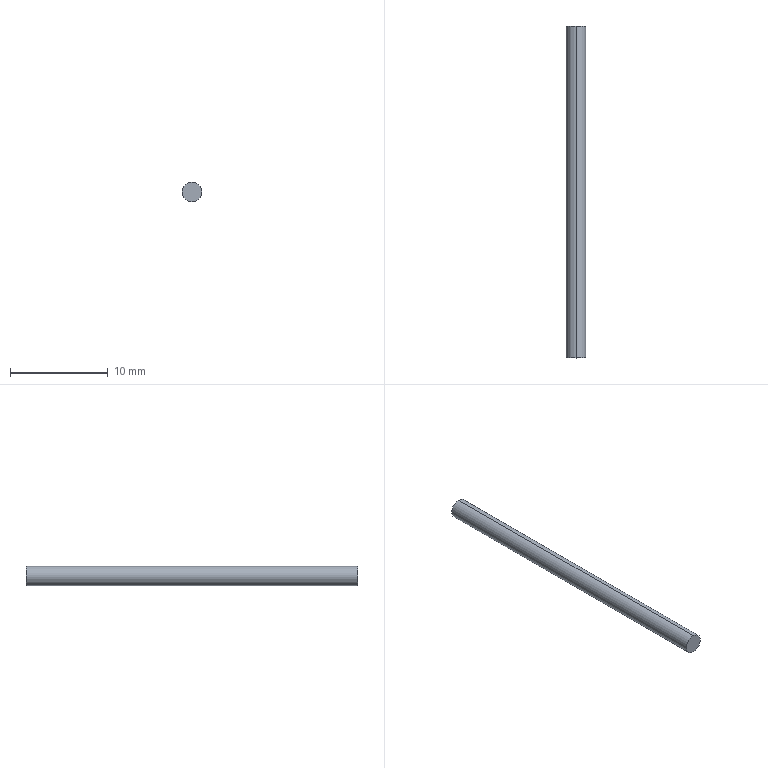Part | SolidWorks | features Extrusion 1 | 1 solid | 4 faces | box 2 x 34 x 2 mm | volume 106.814 mm3 | cylinder 2 | plane 2 | commonest cylinder face diameters 2 x2
STEP:
#1=CARTESIAN_POINT('',(0.,34.,1.));
#2=VERTEX_POINT('',#1);
#3=CARTESIAN_POINT('',(0.,34.,-1.));
#4=VERTEX_POINT('',#3);
#5=CARTESIAN_POINT('',(0.,34.,0.));
#6=DIRECTION('',(0.,1.,0.));
#7=DIRECTION('',(0.,0.,1.));
#8=AXIS2_PLACEMENT_3D('',#5,#6,#7);
#9=CIRCLE('',#8,1.);
#10=EDGE_CURVE('',#2,#4,#9,.T.);
#11=ORIENTED_EDGE('',*,*,#10,.F.);
#12=CARTESIAN_POINT('',(0.,0.,1.));
#13=VERTEX_POINT('',#12);
#14=CARTESIAN_POINT('',(0.,34.,1.));
#15=DIRECTION('',(0.,-1.,0.));
#16=VECTOR('',#15,1000.);
#17=LINE('',#14,#16);
#18=EDGE_CURVE('',#2,#13,#17,.T.);
#19=ORIENTED_EDGE('',*,*,#18,.T.);
#20=CARTESIAN_POINT('',(0.,0.,-1.));
#21=VERTEX_POINT('',#20);
#22=CARTESIAN_POINT('',(0.,0.,0.));
#23=DIRECTION('',(0.,1.,0.));
#24=DIRECTION('',(0.,0.,1.));
#25=AXIS2_PLACEMENT_3D('',#22,#23,#24);
#26=CIRCLE('',#25,1.);
#27=EDGE_CURVE('',#13,#21,#26,.T.);
#28=ORIENTED_EDGE('',*,*,#27,.T.);
#29=CARTESIAN_POINT('',(0.,34.,-1.));
#30=DIRECTION('',(0.,-1.,0.));
#31=VECTOR('',#30,1000.);
#32=LINE('',#29,#31);
#33=EDGE_CURVE('',#4,#21,#32,.T.);
#34=ORIENTED_EDGE('',*,*,#33,.F.);
#35=EDGE_LOOP('',(#11,#19,#28,#34));
#36=FACE_OUTER_BOUND('',#35,.T.);
#37=CARTESIAN_POINT('',(0.,34.,0.));
#38=DIRECTION('',(0.,-1.,0.));
#39=DIRECTION('',(0.,0.,-1.));
#40=AXIS2_PLACEMENT_3D('',#37,#38,#39);
#41=CYLINDRICAL_SURFACE('',#40,1.);
#42=ADVANCED_FACE('',(#36),#41,.T.);
#43=ORIENTED_EDGE('',*,*,#18,.F.);
#44=CARTESIAN_POINT('',(0.,34.,0.));
#45=DIRECTION('',(0.,1.,0.));
#46=DIRECTION('',(0.,0.,1.));
#47=AXIS2_PLACEMENT_3D('',#44,#45,#46);
#48=CIRCLE('',#47,1.);
#49=EDGE_CURVE('',#4,#2,#48,.T.);
#50=ORIENTED_EDGE('',*,*,#49,.F.);
#51=ORIENTED_EDGE('',*,*,#33,.T.);
#52=CARTESIAN_POINT('',(0.,0.,0.));
#53=DIRECTION('',(0.,1.,0.));
#54=DIRECTION('',(0.,0.,1.));
#55=AXIS2_PLACEMENT_3D('',#52,#53,#54);
#56=CIRCLE('',#55,1.);
#57=EDGE_CURVE('',#21,#13,#56,.T.);
#58=ORIENTED_EDGE('',*,*,#57,.T.);
#59=EDGE_LOOP('',(#43,#50,#51,#58));
#60=FACE_OUTER_BOUND('',#59,.T.);
#61=CARTESIAN_POINT('',(0.,34.,0.));
#62=DIRECTION('',(0.,-1.,0.));
#63=DIRECTION('',(0.,0.,-1.));
#64=AXIS2_PLACEMENT_3D('',#61,#62,#63);
#65=CYLINDRICAL_SURFACE('',#64,1.);
#66=ADVANCED_FACE('',(#60),#65,.T.);
#67=ORIENTED_EDGE('',*,*,#49,.T.);
#68=ORIENTED_EDGE('',*,*,#10,.T.);
#69=EDGE_LOOP('',(#67,#68));
#70=FACE_OUTER_BOUND('',#69,.T.);
#71=CARTESIAN_POINT('',(0.,34.,0.));
#72=DIRECTION('',(0.,1.,0.));
#73=DIRECTION('',(0.,0.,1.));
#74=AXIS2_PLACEMENT_3D('',#71,#72,#73);
#75=PLANE('',#74);
#76=ADVANCED_FACE('',(#70),#75,.T.);
#77=ORIENTED_EDGE('',*,*,#57,.F.);
#78=ORIENTED_EDGE('',*,*,#27,.F.);
#79=EDGE_LOOP('',(#77,#78));
#80=FACE_OUTER_BOUND('',#79,.T.);
#81=CARTESIAN_POINT('',(0.,0.,0.));
#82=DIRECTION('',(0.,1.,0.));
#83=DIRECTION('',(0.,0.,1.));
#84=AXIS2_PLACEMENT_3D('',#81,#82,#83);
#85=PLANE('',#84);
#86=ADVANCED_FACE('',(#80),#85,.F.);
#87=CLOSED_SHELL('',(#42,#66,#76,#86));
#88=MANIFOLD_SOLID_BREP('',#87);
#89=CARTESIAN_POINT('',(0.,0.,0.));
#90=DIRECTION('',(0.,0.,1.));
#91=DIRECTION('',(1.,0.,0.));
#92=AXIS2_PLACEMENT_3D('',#89,#90,#91);
#93=(LENGTH_UNIT()NAMED_UNIT(*)SI_UNIT(.MILLI.,.METRE.));
#94=UNCERTAINTY_MEASURE_WITH_UNIT(LENGTH_MEASURE(0.00001),#93,'','');
#95=(NAMED_UNIT(*)PLANE_ANGLE_UNIT()SI_UNIT($,.RADIAN.));
#96=(NAMED_UNIT(*)SI_UNIT($,.STERADIAN.)SOLID_ANGLE_UNIT());
#97=(GEOMETRIC_REPRESENTATION_CONTEXT(3)GLOBAL_UNCERTAINTY_ASSIGNED_CONTEXT((#94))GLOBAL_UNIT_ASSIGNED_CONTEXT((#93,#95,#96))REPRESENTATION_CONTEXT('',''));
#98=ADVANCED_BREP_SHAPE_REPRESENTATION('',(#88,#92),#97);